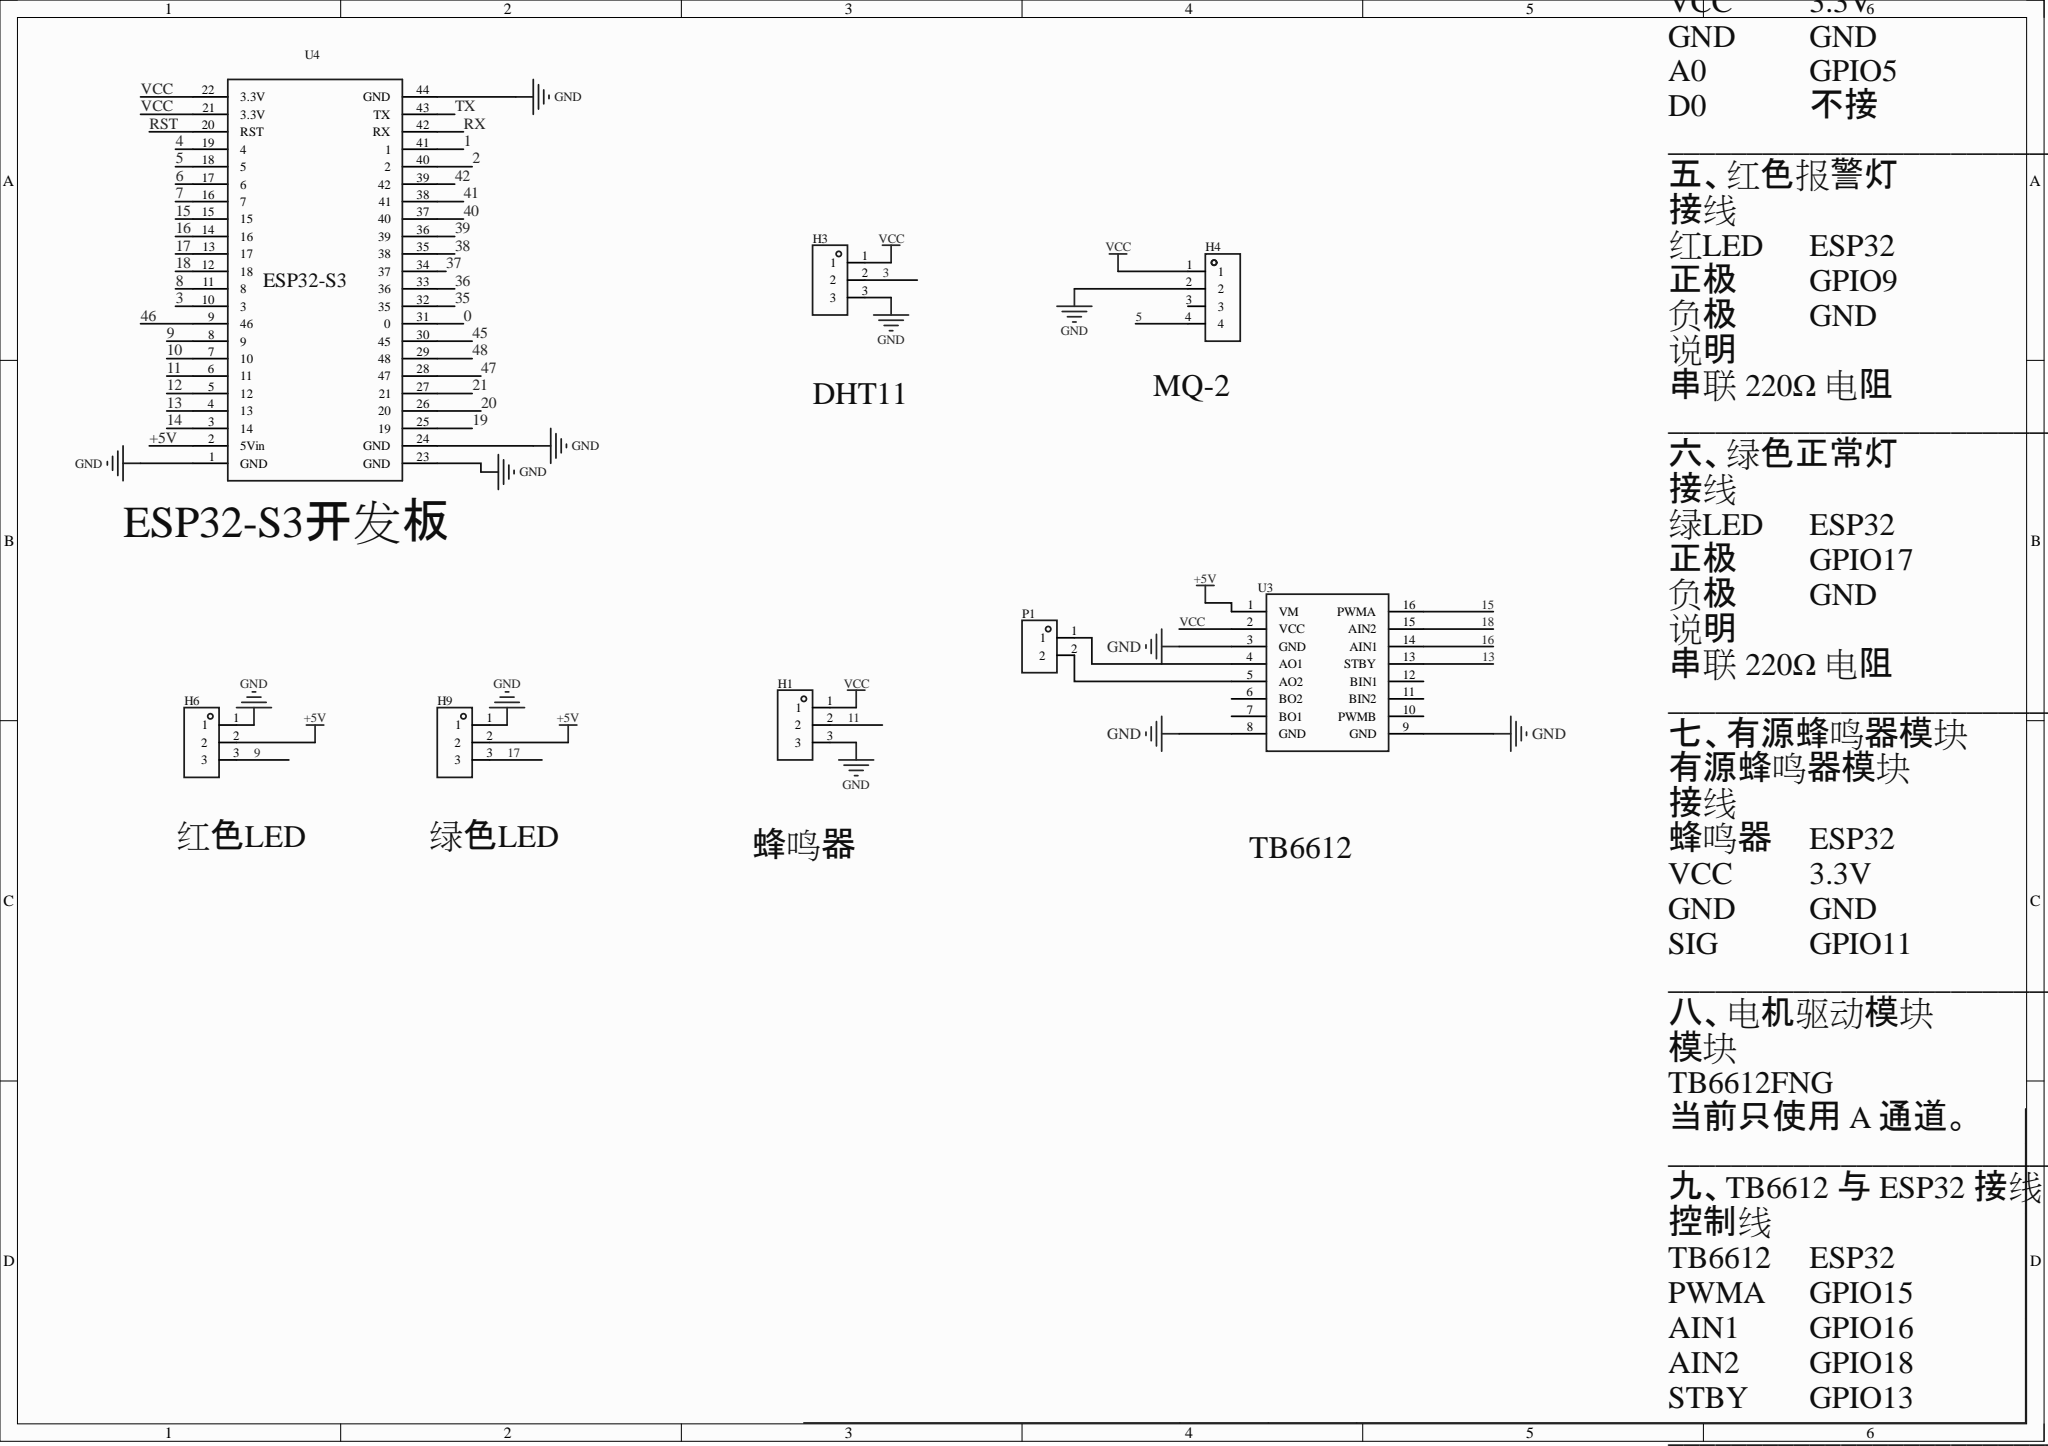Circuit board | Altium Designer | 8 parts | 14 nets
Bill of materials:
Comment,Description,Designator,Footprint,LibRef,Quantity
"","","H1, H3, H6, H9","HDR-TH_3P-P2.54-V-F","HDR-F_2.54_1x3P","4"
"","","H4","HDR-TH_4P-P2.54-V-F","HDR-F_2.54_1x4P","1"
"KF301-2P接线端子","","P1","CONN-TH_XY301V-A-5.0-2P","KF301-2P接线端子","1"
"","","U3","tb6612","tb6612","1"
"NO","","U4","ESP32S3","NO","1"
Netlist (Protel format):
[
H1
HDR-TH_3P-P2.54-V-F




]
[
H3
HDR-TH_3P-P2.54-V-F




]
[
H4
HDR-TH_4P-P2.54-V-F




]
[
H6
HDR-TH_3P-P2.54-V-F




]
[
H9
HDR-TH_3P-P2.54-V-F




]
[
P1
CONN-TH_XY301V-A-5.0-2P
KF301-2P接线端子



]
[
U3
tb6612




]
[
U4
ESP32S3
NO



]
(
VCC
H1-1
H3-1
H4-1
U3-2
U4-21
U4-22
)
(
NetP1_2
P1-2
U3-5
)
(
NetP1_1
P1-1
U3-4
)
(
GND
H1-3
H3-3
H4-2
H6-1
H9-1
U3-3
U3-8
U3-9
U4-1
U4-23
U4-24
U4-44
)
(
+5V
H6-2
H9-2
U3-1
U4-2
)
(
18
U3-15
U4-12
)
(
17
H9-3
U4-13
)
(
16
U3-14
U4-14
)
(
15
U3-16
U4-15
)
(
13
U3-13
U4-4
)
(
11
H1-2
U4-6
)
(
9
H6-3
U4-8
)
(
5
H4-4
U4-18
)
(
3
H3-2
U4-10
)